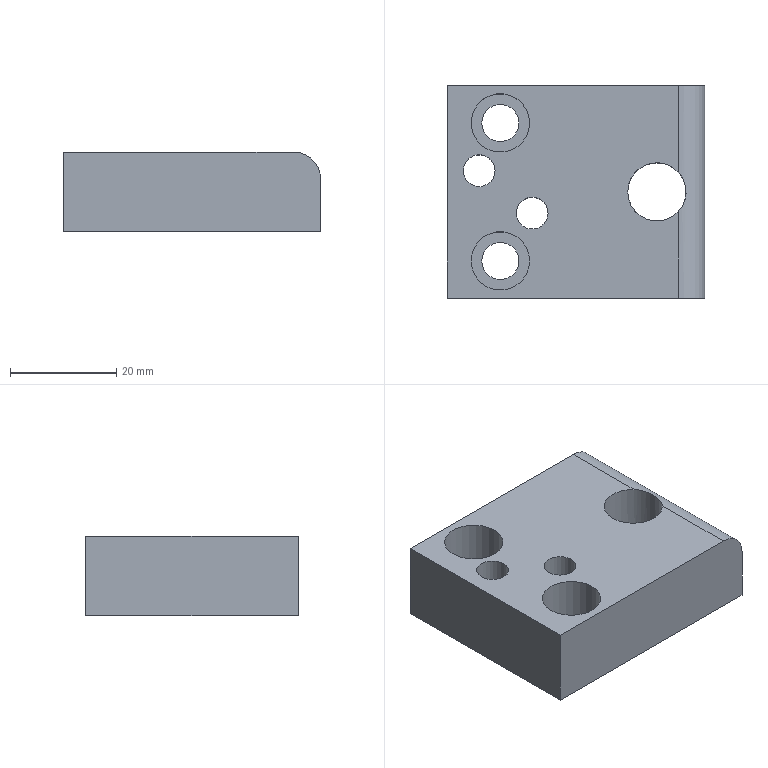Part | NX | features solid 2 | 1 solid | 16 faces | box 48.5 x 40 x 15 mm | volume 24439 mm3 | plane 8 | cylinder 8 | commonest cylinder face diameters 11 x3 6.001 x2 7 x2 10 x1
STEP:
#1=CARTESIAN_POINT('',(614.,-20.,-1.5));
#2=VERTEX_POINT('',#1);
#3=CARTESIAN_POINT('',(570.5,-20.,-1.5));
#4=VERTEX_POINT('',#3);
#5=CARTESIAN_POINT('',(715.,-20.,-1.5));
#6=DIRECTION('',(-1.,0.,0.));
#7=VECTOR('',#6,1000.);
#8=LINE('',#5,#7);
#9=EDGE_CURVE('',#2,#4,#8,.T.);
#10=ORIENTED_EDGE('',*,*,#9,.F.);
#11=CARTESIAN_POINT('',(614.,-3.775,-1.5));
#12=VERTEX_POINT('',#11);
#13=CARTESIAN_POINT('',(614.,0.,-1.5));
#14=DIRECTION('',(0.,1.,0.));
#15=VECTOR('',#14,1000.);
#16=LINE('',#13,#15);
#17=EDGE_CURVE('',#2,#12,#16,.T.);
#18=ORIENTED_EDGE('',*,*,#17,.T.);
#19=CARTESIAN_POINT('',(614.,3.775,-1.5));
#20=VERTEX_POINT('',#19);
#21=CARTESIAN_POINT('',(610.,0.,-1.5));
#22=DIRECTION('',(0.,0.,1.));
#23=DIRECTION('',(-1.,0.,0.));
#24=AXIS2_PLACEMENT_3D('',#21,#22,#23);
#25=CIRCLE('',#24,5.5);
#26=EDGE_CURVE('',#20,#12,#25,.T.);
#27=ORIENTED_EDGE('',*,*,#26,.F.);
#28=CARTESIAN_POINT('',(614.,20.,-1.5));
#29=VERTEX_POINT('',#28);
#30=CARTESIAN_POINT('',(614.,0.,-1.5));
#31=DIRECTION('',(0.,1.,0.));
#32=VECTOR('',#31,1000.);
#33=LINE('',#30,#32);
#34=EDGE_CURVE('',#20,#29,#33,.T.);
#35=ORIENTED_EDGE('',*,*,#34,.T.);
#36=CARTESIAN_POINT('',(570.5,20.,-1.5));
#37=VERTEX_POINT('',#36);
#38=CARTESIAN_POINT('',(715.,20.,-1.5));
#39=DIRECTION('',(1.,0.,0.));
#40=VECTOR('',#39,1000.);
#41=LINE('',#38,#40);
#42=EDGE_CURVE('',#37,#29,#41,.T.);
#43=ORIENTED_EDGE('',*,*,#42,.F.);
#44=CARTESIAN_POINT('',(570.5,0.,-1.5));
#45=DIRECTION('',(0.,1.,0.));
#46=VECTOR('',#45,1000.);
#47=LINE('',#44,#46);
#48=EDGE_CURVE('',#4,#37,#47,.T.);
#49=ORIENTED_EDGE('',*,*,#48,.F.);
#50=EDGE_LOOP('',(#10,#18,#27,#35,#43,#49));
#51=FACE_BOUND('',#50,.T.);
#52=CARTESIAN_POINT('',(573.5,4.,-1.5));
#53=VERTEX_POINT('',#52);
#54=CARTESIAN_POINT('',(576.5,4.,-1.5));
#55=DIRECTION('',(0.,0.,1.));
#56=DIRECTION('',(-1.,0.,0.));
#57=AXIS2_PLACEMENT_3D('',#54,#55,#56);
#58=CIRCLE('',#57,3.001);
#59=EDGE_CURVE('',#53,#53,#58,.T.);
#60=ORIENTED_EDGE('',*,*,#59,.F.);
#61=EDGE_LOOP('',(#60));
#62=FACE_BOUND('',#61,.T.);
#63=CARTESIAN_POINT('',(583.5,-4.,-1.5));
#64=VERTEX_POINT('',#63);
#65=CARTESIAN_POINT('',(586.5,-4.,-1.5));
#66=DIRECTION('',(0.,0.,1.));
#67=DIRECTION('',(-1.,0.,0.));
#68=AXIS2_PLACEMENT_3D('',#65,#66,#67);
#69=CIRCLE('',#68,3.001);
#70=EDGE_CURVE('',#64,#64,#69,.T.);
#71=ORIENTED_EDGE('',*,*,#70,.F.);
#72=EDGE_LOOP('',(#71));
#73=FACE_BOUND('',#72,.T.);
#74=CARTESIAN_POINT('',(575.,13.,-1.5));
#75=VERTEX_POINT('',#74);
#76=CARTESIAN_POINT('',(580.5,13.,-1.5));
#77=DIRECTION('',(0.,0.,1.));
#78=DIRECTION('',(-1.,0.,0.));
#79=AXIS2_PLACEMENT_3D('',#76,#77,#78);
#80=CIRCLE('',#79,5.5);
#81=EDGE_CURVE('',#75,#75,#80,.T.);
#82=ORIENTED_EDGE('',*,*,#81,.F.);
#83=EDGE_LOOP('',(#82));
#84=FACE_BOUND('',#83,.T.);
#85=CARTESIAN_POINT('',(575.,-13.,-1.5));
#86=VERTEX_POINT('',#85);
#87=CARTESIAN_POINT('',(580.5,-13.,-1.5));
#88=DIRECTION('',(0.,0.,-1.));
#89=DIRECTION('',(-1.,0.,0.));
#90=AXIS2_PLACEMENT_3D('',#87,#88,#89);
#91=CIRCLE('',#90,5.5);
#92=EDGE_CURVE('',#86,#86,#91,.T.);
#93=ORIENTED_EDGE('',*,*,#92,.T.);
#94=EDGE_LOOP('',(#93));
#95=FACE_BOUND('',#94,.T.);
#96=CARTESIAN_POINT('',(715.,0.,-1.5));
#97=DIRECTION('',(0.,0.,1.));
#98=DIRECTION('',(-1.,0.,0.));
#99=AXIS2_PLACEMENT_3D('',#96,#97,#98);
#100=PLANE('',#99);
#101=ADVANCED_FACE('',(#51,#62,#73,#84,#95),#100,.T.);
#102=CARTESIAN_POINT('',(619.,20.,-6.5));
#103=VERTEX_POINT('',#102);
#104=CARTESIAN_POINT('',(619.,20.,-16.5));
#105=VERTEX_POINT('',#104);
#106=CARTESIAN_POINT('',(619.,20.,-51.5));
#107=DIRECTION('',(0.,0.,-1.));
#108=VECTOR('',#107,1000.);
#109=LINE('',#106,#108);
#110=EDGE_CURVE('',#103,#105,#109,.T.);
#111=ORIENTED_EDGE('',*,*,#110,.F.);
#112=CARTESIAN_POINT('',(619.,-20.,-6.5));
#113=VERTEX_POINT('',#112);
#114=CARTESIAN_POINT('',(619.,29.,-6.5));
#115=DIRECTION('',(0.,1.,0.));
#116=VECTOR('',#115,1000.);
#117=LINE('',#114,#116);
#118=EDGE_CURVE('',#103,#113,#117,.F.);
#119=ORIENTED_EDGE('',*,*,#118,.T.);
#120=CARTESIAN_POINT('',(619.,-20.,-16.5));
#121=VERTEX_POINT('',#120);
#122=CARTESIAN_POINT('',(619.,-20.,-51.5));
#123=DIRECTION('',(0.,0.,1.));
#124=VECTOR('',#123,1000.);
#125=LINE('',#122,#124);
#126=EDGE_CURVE('',#121,#113,#125,.T.);
#127=ORIENTED_EDGE('',*,*,#126,.F.);
#128=CARTESIAN_POINT('',(619.,0.,-16.5));
#129=DIRECTION('',(0.,-1.,0.));
#130=VECTOR('',#129,1000.);
#131=LINE('',#128,#130);
#132=EDGE_CURVE('',#105,#121,#131,.T.);
#133=ORIENTED_EDGE('',*,*,#132,.F.);
#134=EDGE_LOOP('',(#111,#119,#127,#133));
#135=FACE_BOUND('',#134,.T.);
#136=CARTESIAN_POINT('',(619.,29.,0.));
#137=DIRECTION('',(1.,0.,0.));
#138=DIRECTION('',(0.,0.,1.));
#139=AXIS2_PLACEMENT_3D('',#136,#137,#138);
#140=PLANE('',#139);
#141=ADVANCED_FACE('',(#135),#140,.T.);
#142=ORIENTED_EDGE('',*,*,#126,.T.);
#143=CARTESIAN_POINT('',(614.,-20.,-6.5));
#144=DIRECTION('',(0.,-1.,0.));
#145=DIRECTION('',(0.,0.,-1.));
#146=AXIS2_PLACEMENT_3D('',#143,#144,#145);
#147=CIRCLE('',#146,5.);
#148=EDGE_CURVE('',#113,#2,#147,.T.);
#149=ORIENTED_EDGE('',*,*,#148,.T.);
#150=ORIENTED_EDGE('',*,*,#9,.T.);
#151=CARTESIAN_POINT('',(570.5,-20.,-16.5));
#152=VERTEX_POINT('',#151);
#153=CARTESIAN_POINT('',(570.5,-20.,-51.5));
#154=DIRECTION('',(0.,0.,1.));
#155=VECTOR('',#154,1000.);
#156=LINE('',#153,#155);
#157=EDGE_CURVE('',#152,#4,#156,.T.);
#158=ORIENTED_EDGE('',*,*,#157,.F.);
#159=CARTESIAN_POINT('',(715.,-20.,-16.5));
#160=DIRECTION('',(1.,0.,0.));
#161=VECTOR('',#160,1000.);
#162=LINE('',#159,#161);
#163=EDGE_CURVE('',#152,#121,#162,.T.);
#164=ORIENTED_EDGE('',*,*,#163,.T.);
#165=EDGE_LOOP('',(#142,#149,#150,#158,#164));
#166=FACE_BOUND('',#165,.T.);
#167=CARTESIAN_POINT('',(715.,-20.,-51.5));
#168=DIRECTION('',(0.,-1.,0.));
#169=DIRECTION('',(0.,0.,1.));
#170=AXIS2_PLACEMENT_3D('',#167,#168,#169);
#171=PLANE('',#170);
#172=ADVANCED_FACE('',(#166),#171,.T.);
#173=ORIENTED_EDGE('',*,*,#42,.T.);
#174=CARTESIAN_POINT('',(614.,20.,-6.5));
#175=DIRECTION('',(0.,1.,0.));
#176=DIRECTION('',(0.,0.,1.));
#177=AXIS2_PLACEMENT_3D('',#174,#175,#176);
#178=CIRCLE('',#177,5.);
#179=EDGE_CURVE('',#29,#103,#178,.T.);
#180=ORIENTED_EDGE('',*,*,#179,.T.);
#181=ORIENTED_EDGE('',*,*,#110,.T.);
#182=CARTESIAN_POINT('',(570.5,20.,-16.5));
#183=VERTEX_POINT('',#182);
#184=CARTESIAN_POINT('',(715.,20.,-16.5));
#185=DIRECTION('',(-1.,0.,0.));
#186=VECTOR('',#185,1000.);
#187=LINE('',#184,#186);
#188=EDGE_CURVE('',#105,#183,#187,.T.);
#189=ORIENTED_EDGE('',*,*,#188,.T.);
#190=CARTESIAN_POINT('',(570.5,20.,-51.5));
#191=DIRECTION('',(0.,0.,1.));
#192=VECTOR('',#191,1000.);
#193=LINE('',#190,#192);
#194=EDGE_CURVE('',#183,#37,#193,.T.);
#195=ORIENTED_EDGE('',*,*,#194,.T.);
#196=EDGE_LOOP('',(#173,#180,#181,#189,#195));
#197=FACE_BOUND('',#196,.T.);
#198=CARTESIAN_POINT('',(715.,20.,-51.5));
#199=DIRECTION('',(0.,1.,0.));
#200=DIRECTION('',(0.,0.,-1.));
#201=AXIS2_PLACEMENT_3D('',#198,#199,#200);
#202=PLANE('',#201);
#203=ADVANCED_FACE('',(#197),#202,.T.);
#204=CARTESIAN_POINT('',(615.5,0.,-16.5));
#205=VERTEX_POINT('',#204);
#206=CARTESIAN_POINT('',(610.,0.,-16.5));
#207=DIRECTION('',(0.,0.,-1.));
#208=DIRECTION('',(1.,0.,0.));
#209=AXIS2_PLACEMENT_3D('',#206,#207,#208);
#210=CIRCLE('',#209,5.5);
#211=EDGE_CURVE('',#205,#205,#210,.T.);
#212=ORIENTED_EDGE('',*,*,#211,.F.);
#213=EDGE_LOOP('',(#212));
#214=FACE_BOUND('',#213,.T.);
#215=CARTESIAN_POINT('',(579.5,4.,-16.5));
#216=VERTEX_POINT('',#215);
#217=CARTESIAN_POINT('',(576.5,4.,-16.5));
#218=DIRECTION('',(0.,0.,-1.));
#219=DIRECTION('',(1.,0.,0.));
#220=AXIS2_PLACEMENT_3D('',#217,#218,#219);
#221=CIRCLE('',#220,3.001);
#222=EDGE_CURVE('',#216,#216,#221,.T.);
#223=ORIENTED_EDGE('',*,*,#222,.F.);
#224=EDGE_LOOP('',(#223));
#225=FACE_BOUND('',#224,.T.);
#226=CARTESIAN_POINT('',(589.5,-4.,-16.5));
#227=VERTEX_POINT('',#226);
#228=CARTESIAN_POINT('',(586.5,-4.,-16.5));
#229=DIRECTION('',(0.,0.,-1.));
#230=DIRECTION('',(1.,0.,0.));
#231=AXIS2_PLACEMENT_3D('',#228,#229,#230);
#232=CIRCLE('',#231,3.001);
#233=EDGE_CURVE('',#227,#227,#232,.T.);
#234=ORIENTED_EDGE('',*,*,#233,.F.);
#235=EDGE_LOOP('',(#234));
#236=FACE_BOUND('',#235,.T.);
#237=CARTESIAN_POINT('',(584.,13.,-16.5));
#238=VERTEX_POINT('',#237);
#239=CARTESIAN_POINT('',(580.5,13.,-16.5));
#240=DIRECTION('',(0.,0.,-1.));
#241=DIRECTION('',(1.,0.,0.));
#242=AXIS2_PLACEMENT_3D('',#239,#240,#241);
#243=CIRCLE('',#242,3.5);
#244=EDGE_CURVE('',#238,#238,#243,.T.);
#245=ORIENTED_EDGE('',*,*,#244,.F.);
#246=EDGE_LOOP('',(#245));
#247=FACE_BOUND('',#246,.T.);
#248=CARTESIAN_POINT('',(584.,-13.,-16.5));
#249=VERTEX_POINT('',#248);
#250=CARTESIAN_POINT('',(580.5,-13.,-16.5));
#251=DIRECTION('',(0.,0.,-1.));
#252=DIRECTION('',(1.,0.,0.));
#253=AXIS2_PLACEMENT_3D('',#250,#251,#252);
#254=CIRCLE('',#253,3.5);
#255=EDGE_CURVE('',#249,#249,#254,.T.);
#256=ORIENTED_EDGE('',*,*,#255,.F.);
#257=EDGE_LOOP('',(#256));
#258=FACE_BOUND('',#257,.T.);
#259=ORIENTED_EDGE('',*,*,#188,.F.);
#260=ORIENTED_EDGE('',*,*,#132,.T.);
#261=ORIENTED_EDGE('',*,*,#163,.F.);
#262=CARTESIAN_POINT('',(570.5,0.,-16.5));
#263=DIRECTION('',(0.,-1.,0.));
#264=VECTOR('',#263,1000.);
#265=LINE('',#262,#264);
#266=EDGE_CURVE('',#183,#152,#265,.T.);
#267=ORIENTED_EDGE('',*,*,#266,.F.);
#268=EDGE_LOOP('',(#259,#260,#261,#267));
#269=FACE_BOUND('',#268,.T.);
#270=CARTESIAN_POINT('',(694.,0.,-16.5));
#271=DIRECTION('',(0.,0.,-1.));
#272=DIRECTION('',(1.,0.,0.));
#273=AXIS2_PLACEMENT_3D('',#270,#271,#272);
#274=PLANE('',#273);
#275=ADVANCED_FACE('',(#214,#225,#236,#247,#258,#269),#274,.T.);
#276=ORIENTED_EDGE('',*,*,#194,.F.);
#277=ORIENTED_EDGE('',*,*,#266,.T.);
#278=ORIENTED_EDGE('',*,*,#157,.T.);
#279=ORIENTED_EDGE('',*,*,#48,.T.);
#280=EDGE_LOOP('',(#276,#277,#278,#279));
#281=FACE_BOUND('',#280,.T.);
#282=CARTESIAN_POINT('',(570.5,0.,-51.5));
#283=DIRECTION('',(-1.,0.,0.));
#284=DIRECTION('',(0.,0.,-1.));
#285=AXIS2_PLACEMENT_3D('',#282,#283,#284);
#286=PLANE('',#285);
#287=ADVANCED_FACE('',(#281),#286,.T.);
#288=ORIENTED_EDGE('',*,*,#255,.T.);
#289=EDGE_LOOP('',(#288));
#290=FACE_BOUND('',#289,.T.);
#291=CARTESIAN_POINT('',(584.,-13.,-10.5));
#292=VERTEX_POINT('',#291);
#293=CARTESIAN_POINT('',(580.5,-13.,-10.5));
#294=DIRECTION('',(0.,0.,-1.));
#295=DIRECTION('',(1.,0.,0.));
#296=AXIS2_PLACEMENT_3D('',#293,#294,#295);
#297=CIRCLE('',#296,3.5);
#298=EDGE_CURVE('',#292,#292,#297,.T.);
#299=ORIENTED_EDGE('',*,*,#298,.F.);
#300=EDGE_LOOP('',(#299));
#301=FACE_BOUND('',#300,.T.);
#302=CARTESIAN_POINT('',(580.5,-13.,0.5));
#303=DIRECTION('',(0.,0.,-1.));
#304=DIRECTION('',(-1.,0.,0.));
#305=AXIS2_PLACEMENT_3D('',#302,#303,#304);
#306=CYLINDRICAL_SURFACE('',#305,3.5);
#307=ADVANCED_FACE('',(#290,#301),#306,.F.);
#308=ORIENTED_EDGE('',*,*,#298,.T.);
#309=EDGE_LOOP('',(#308));
#310=FACE_BOUND('',#309,.T.);
#311=CARTESIAN_POINT('',(575.,-13.,-10.5));
#312=VERTEX_POINT('',#311);
#313=CARTESIAN_POINT('',(580.5,-13.,-10.5));
#314=DIRECTION('',(0.,0.,1.));
#315=DIRECTION('',(-1.,0.,0.));
#316=AXIS2_PLACEMENT_3D('',#313,#314,#315);
#317=CIRCLE('',#316,5.5);
#318=EDGE_CURVE('',#312,#312,#317,.F.);
#319=ORIENTED_EDGE('',*,*,#318,.F.);
#320=EDGE_LOOP('',(#319));
#321=FACE_BOUND('',#320,.T.);
#322=CARTESIAN_POINT('',(580.5,-13.,-10.5));
#323=DIRECTION('',(0.,0.,-1.));
#324=DIRECTION('',(1.,0.,0.));
#325=AXIS2_PLACEMENT_3D('',#322,#323,#324);
#326=PLANE('',#325);
#327=ADVANCED_FACE('',(#310,#321),#326,.F.);
#328=ORIENTED_EDGE('',*,*,#318,.T.);
#329=EDGE_LOOP('',(#328));
#330=FACE_BOUND('',#329,.T.);
#331=ORIENTED_EDGE('',*,*,#92,.F.);
#332=EDGE_LOOP('',(#331));
#333=FACE_BOUND('',#332,.T.);
#334=CARTESIAN_POINT('',(580.5,-13.,-1.5));
#335=DIRECTION('',(0.,0.,-1.));
#336=DIRECTION('',(-1.,0.,0.));
#337=AXIS2_PLACEMENT_3D('',#334,#335,#336);
#338=CYLINDRICAL_SURFACE('',#337,5.5);
#339=ADVANCED_FACE('',(#330,#333),#338,.F.);
#340=ORIENTED_EDGE('',*,*,#244,.T.);
#341=EDGE_LOOP('',(#340));
#342=FACE_BOUND('',#341,.T.);
#343=CARTESIAN_POINT('',(584.,13.,-10.5));
#344=VERTEX_POINT('',#343);
#345=CARTESIAN_POINT('',(580.5,13.,-10.5));
#346=DIRECTION('',(0.,0.,1.));
#347=DIRECTION('',(1.,0.,0.));
#348=AXIS2_PLACEMENT_3D('',#345,#346,#347);
#349=CIRCLE('',#348,3.5);
#350=EDGE_CURVE('',#344,#344,#349,.T.);
#351=ORIENTED_EDGE('',*,*,#350,.T.);
#352=EDGE_LOOP('',(#351));
#353=FACE_BOUND('',#352,.T.);
#354=CARTESIAN_POINT('',(580.5,13.,0.5));
#355=DIRECTION('',(0.,0.,-1.));
#356=DIRECTION('',(-1.,0.,0.));
#357=AXIS2_PLACEMENT_3D('',#354,#355,#356);
#358=CYLINDRICAL_SURFACE('',#357,3.5);
#359=ADVANCED_FACE('',(#342,#353),#358,.F.);
#360=ORIENTED_EDGE('',*,*,#350,.F.);
#361=EDGE_LOOP('',(#360));
#362=FACE_BOUND('',#361,.T.);
#363=CARTESIAN_POINT('',(575.,13.,-10.5));
#364=VERTEX_POINT('',#363);
#365=CARTESIAN_POINT('',(580.5,13.,-10.5));
#366=DIRECTION('',(0.,0.,-1.));
#367=DIRECTION('',(-1.,0.,0.));
#368=AXIS2_PLACEMENT_3D('',#365,#366,#367);
#369=CIRCLE('',#368,5.5);
#370=EDGE_CURVE('',#364,#364,#369,.F.);
#371=ORIENTED_EDGE('',*,*,#370,.T.);
#372=EDGE_LOOP('',(#371));
#373=FACE_BOUND('',#372,.T.);
#374=CARTESIAN_POINT('',(580.5,13.,-10.5));
#375=DIRECTION('',(0.,0.,-1.));
#376=DIRECTION('',(1.,0.,0.));
#377=AXIS2_PLACEMENT_3D('',#374,#375,#376);
#378=PLANE('',#377);
#379=ADVANCED_FACE('',(#362,#373),#378,.F.);
#380=ORIENTED_EDGE('',*,*,#370,.F.);
#381=EDGE_LOOP('',(#380));
#382=FACE_BOUND('',#381,.T.);
#383=ORIENTED_EDGE('',*,*,#81,.T.);
#384=EDGE_LOOP('',(#383));
#385=FACE_BOUND('',#384,.T.);
#386=CARTESIAN_POINT('',(580.5,13.,-1.5));
#387=DIRECTION('',(0.,0.,-1.));
#388=DIRECTION('',(-1.,0.,0.));
#389=AXIS2_PLACEMENT_3D('',#386,#387,#388);
#390=CYLINDRICAL_SURFACE('',#389,5.5);
#391=ADVANCED_FACE('',(#382,#385),#390,.F.);
#392=ORIENTED_EDGE('',*,*,#70,.T.);
#393=EDGE_LOOP('',(#392));
#394=FACE_BOUND('',#393,.T.);
#395=ORIENTED_EDGE('',*,*,#233,.T.);
#396=EDGE_LOOP('',(#395));
#397=FACE_BOUND('',#396,.T.);
#398=CARTESIAN_POINT('',(586.5,-4.,0.5));
#399=DIRECTION('',(0.,0.,-1.));
#400=DIRECTION('',(1.,0.,0.));
#401=AXIS2_PLACEMENT_3D('',#398,#399,#400);
#402=CYLINDRICAL_SURFACE('',#401,3.001);
#403=ADVANCED_FACE('',(#394,#397),#402,.F.);
#404=ORIENTED_EDGE('',*,*,#59,.T.);
#405=EDGE_LOOP('',(#404));
#406=FACE_BOUND('',#405,.T.);
#407=ORIENTED_EDGE('',*,*,#222,.T.);
#408=EDGE_LOOP('',(#407));
#409=FACE_BOUND('',#408,.T.);
#410=CARTESIAN_POINT('',(576.5,4.,0.5));
#411=DIRECTION('',(0.,0.,-1.));
#412=DIRECTION('',(-1.,0.,0.));
#413=AXIS2_PLACEMENT_3D('',#410,#411,#412);
#414=CYLINDRICAL_SURFACE('',#413,3.001);
#415=ADVANCED_FACE('',(#406,#409),#414,.F.);
#416=ORIENTED_EDGE('',*,*,#26,.T.);
#417=CARTESIAN_POINT('',(614.,-3.775,-1.5));
#418=CARTESIAN_POINT('',(614.963,-2.755,-1.5));
#419=CARTESIAN_POINT('',(616.037,-0.004291,-1.961));
#420=CARTESIAN_POINT('',(614.962,2.755,-1.5));
#421=CARTESIAN_POINT('',(614.,3.775,-1.5));
#422=B_SPLINE_CURVE_WITH_KNOTS('',3,(#417,#418,#419,#420,#421),.UNSPECIFIED.,.F.,.F.,(4,1,4),(0.,0.004144,0.008289),.UNSPECIFIED.);
#423=EDGE_CURVE('',#12,#20,#422,.T.);
#424=ORIENTED_EDGE('',*,*,#423,.T.);
#425=EDGE_LOOP('',(#416,#424));
#426=FACE_BOUND('',#425,.T.);
#427=ORIENTED_EDGE('',*,*,#211,.T.);
#428=EDGE_LOOP('',(#427));
#429=FACE_BOUND('',#428,.T.);
#430=CARTESIAN_POINT('',(610.,0.,-34.5));
#431=DIRECTION('',(0.,0.,1.));
#432=DIRECTION('',(-1.,0.,0.));
#433=AXIS2_PLACEMENT_3D('',#430,#431,#432);
#434=CYLINDRICAL_SURFACE('',#433,5.5);
#435=ADVANCED_FACE('',(#426,#429),#434,.F.);
#436=ORIENTED_EDGE('',*,*,#148,.F.);
#437=ORIENTED_EDGE('',*,*,#118,.F.);
#438=ORIENTED_EDGE('',*,*,#179,.F.);
#439=ORIENTED_EDGE('',*,*,#34,.F.);
#440=ORIENTED_EDGE('',*,*,#423,.F.);
#441=ORIENTED_EDGE('',*,*,#17,.F.);
#442=EDGE_LOOP('',(#436,#437,#438,#439,#440,#441));
#443=FACE_BOUND('',#442,.T.);
#444=CARTESIAN_POINT('',(614.,0.,-6.5));
#445=DIRECTION('',(0.,1.,0.));
#446=DIRECTION('',(0.,0.,1.));
#447=AXIS2_PLACEMENT_3D('',#444,#445,#446);
#448=CYLINDRICAL_SURFACE('',#447,5.);
#449=ADVANCED_FACE('',(#443),#448,.T.);
#450=CLOSED_SHELL('',(#101,#141,#172,#203,#275,#287,#307,#327,#339,#359,#379,#391,#403,#415,#435,#449));
#451=MANIFOLD_SOLID_BREP('',#450);
#452=(LENGTH_UNIT()NAMED_UNIT(*)SI_UNIT(.MILLI.,.METRE.));
#453=UNCERTAINTY_MEASURE_WITH_UNIT(LENGTH_MEASURE(0.0508),#452,'','');
#454=(NAMED_UNIT(*)PLANE_ANGLE_UNIT()SI_UNIT($,.RADIAN.));
#455=(NAMED_UNIT(*)SI_UNIT($,.STERADIAN.)SOLID_ANGLE_UNIT());
#456=(GEOMETRIC_REPRESENTATION_CONTEXT(3)GLOBAL_UNCERTAINTY_ASSIGNED_CONTEXT((#453))GLOBAL_UNIT_ASSIGNED_CONTEXT((#452,#454,#455))REPRESENTATION_CONTEXT('',''));
#457=ADVANCED_BREP_SHAPE_REPRESENTATION('',(#451),#456);